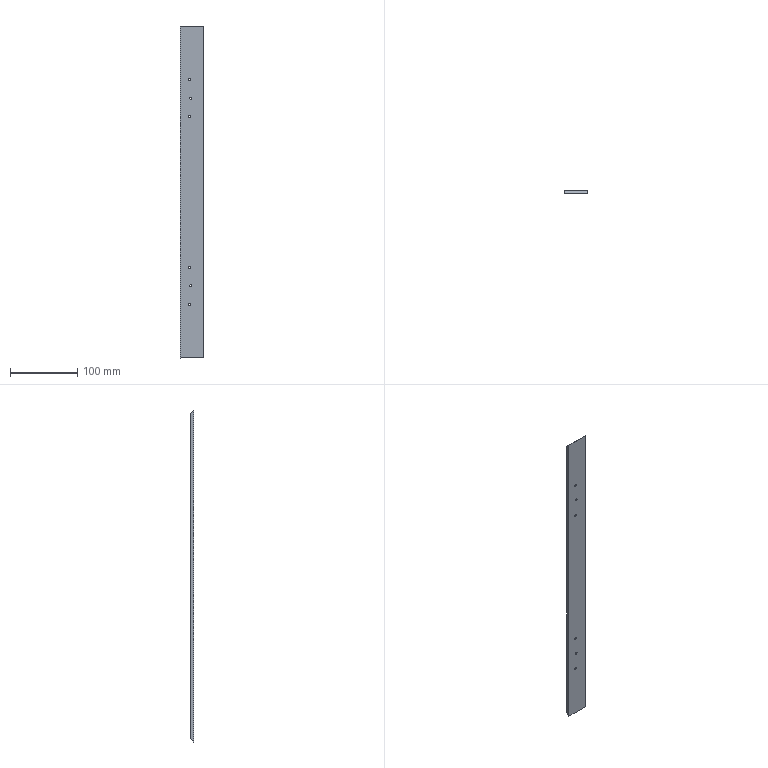Part | STEP file | 09-28 Cover side plate 4 | 1 solid | 18 faces | box 35 x 5 x 495 mm | volume 85493 mm3 | cylinder 12 | plane 6 | commonest cylinder face diameters 3.3 x12